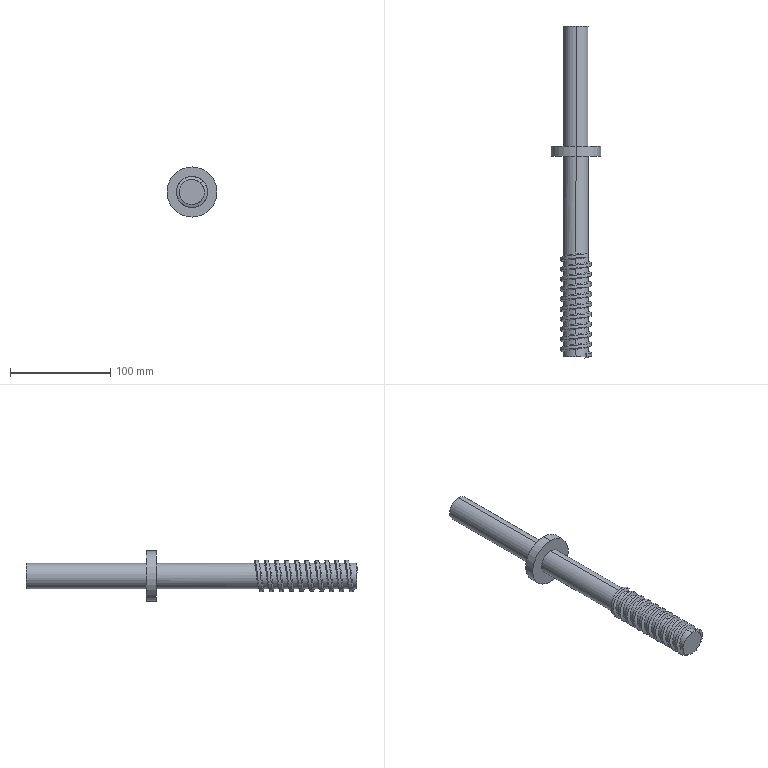Part | SolidWorks | features ICE 2, Extrusion 1, Helix 1, HoleWzd 1, Sweep 1 | 1 solid | 40 faces | box 50 x 331.25 x 50 mm | volume 179506 mm3 | cylinder 28 | plane 6 | spline 4 | cone 2 | commonest cylinder face diameters 25 x24 17.5 x2 50 x2